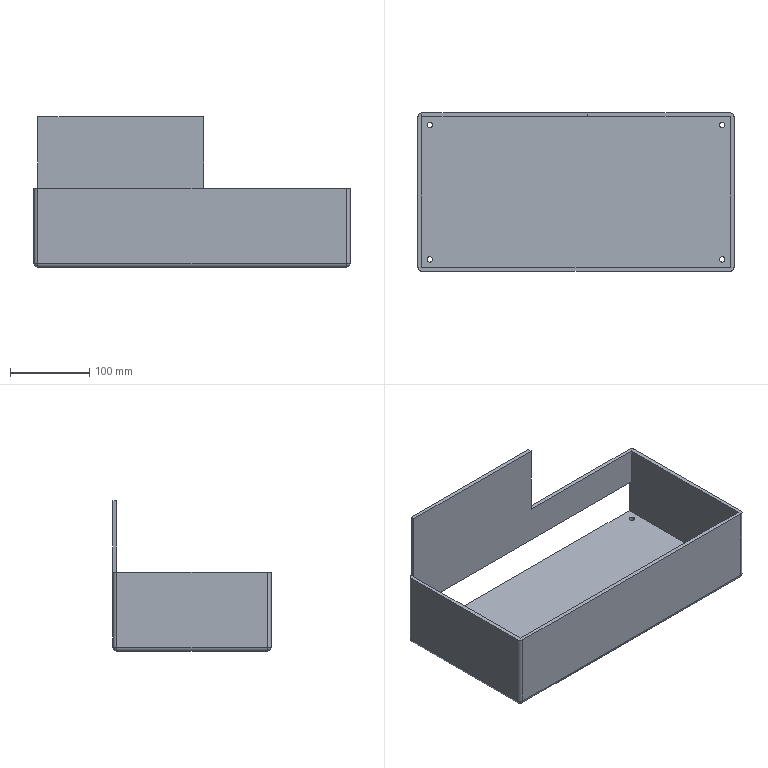Part | SolidWorks | features ICE 3, Fillet 2, Extrusion 1, Shell 1 | 1 solid | 35 faces | box 400 x 200 x 190 mm | volume 953105 mm3 | cylinder 16 | plane 15 | sphere 4 | commonest cylinder face diameters 7 x8 10 x8
STEP:
#1=CARTESIAN_POINT('',(-188.5,-85.,0.));
#2=VERTEX_POINT('',#1);
#3=CARTESIAN_POINT('',(-181.5,-85.,0.));
#4=VERTEX_POINT('',#3);
#5=CARTESIAN_POINT('',(-185.,-85.,0.));
#6=DIRECTION('',(0.,0.,1.));
#7=DIRECTION('',(1.,0.,0.));
#8=AXIS2_PLACEMENT_3D('',#5,#6,#7);
#9=CIRCLE('',#8,3.5);
#10=EDGE_CURVE('',#2,#4,#9,.T.);
#11=ORIENTED_EDGE('',*,*,#10,.F.);
#12=CARTESIAN_POINT('',(-188.5,-85.,5.));
#13=VERTEX_POINT('',#12);
#14=CARTESIAN_POINT('',(-188.5,-85.,-55.));
#15=DIRECTION('',(0.,0.,1.));
#16=VECTOR('',#15,1000.);
#17=LINE('',#14,#16);
#18=EDGE_CURVE('',#2,#13,#17,.T.);
#19=ORIENTED_EDGE('',*,*,#18,.T.);
#20=CARTESIAN_POINT('',(-181.5,-85.,5.));
#21=VERTEX_POINT('',#20);
#22=CARTESIAN_POINT('',(-185.,-85.,5.));
#23=DIRECTION('',(0.,0.,1.));
#24=DIRECTION('',(-1.,0.,0.));
#25=AXIS2_PLACEMENT_3D('',#22,#23,#24);
#26=CIRCLE('',#25,3.5);
#27=EDGE_CURVE('',#13,#21,#26,.T.);
#28=ORIENTED_EDGE('',*,*,#27,.T.);
#29=CARTESIAN_POINT('',(-181.5,-85.,-55.));
#30=DIRECTION('',(0.,0.,1.));
#31=VECTOR('',#30,1000.);
#32=LINE('',#29,#31);
#33=EDGE_CURVE('',#4,#21,#32,.T.);
#34=ORIENTED_EDGE('',*,*,#33,.F.);
#35=EDGE_LOOP('',(#11,#19,#28,#34));
#36=FACE_OUTER_BOUND('',#35,.T.);
#37=CARTESIAN_POINT('',(-185.,-85.,-55.));
#38=DIRECTION('',(0.,0.,1.));
#39=DIRECTION('',(1.,0.,0.));
#40=AXIS2_PLACEMENT_3D('',#37,#38,#39);
#41=CYLINDRICAL_SURFACE('',#40,3.5);
#42=ADVANCED_FACE('',(#36),#41,.F.);
#43=CARTESIAN_POINT('',(181.5,-85.,0.));
#44=VERTEX_POINT('',#43);
#45=CARTESIAN_POINT('',(188.5,-85.,0.));
#46=VERTEX_POINT('',#45);
#47=CARTESIAN_POINT('',(185.,-85.,0.));
#48=DIRECTION('',(0.,0.,1.));
#49=DIRECTION('',(1.,0.,0.));
#50=AXIS2_PLACEMENT_3D('',#47,#48,#49);
#51=CIRCLE('',#50,3.5);
#52=EDGE_CURVE('',#44,#46,#51,.T.);
#53=ORIENTED_EDGE('',*,*,#52,.F.);
#54=CARTESIAN_POINT('',(181.5,-85.,5.));
#55=VERTEX_POINT('',#54);
#56=CARTESIAN_POINT('',(181.5,-85.,-55.));
#57=DIRECTION('',(0.,0.,1.));
#58=VECTOR('',#57,1000.);
#59=LINE('',#56,#58);
#60=EDGE_CURVE('',#44,#55,#59,.T.);
#61=ORIENTED_EDGE('',*,*,#60,.T.);
#62=CARTESIAN_POINT('',(188.5,-85.,5.));
#63=VERTEX_POINT('',#62);
#64=CARTESIAN_POINT('',(185.,-85.,5.));
#65=DIRECTION('',(0.,0.,1.));
#66=DIRECTION('',(1.,0.,0.));
#67=AXIS2_PLACEMENT_3D('',#64,#65,#66);
#68=CIRCLE('',#67,3.5);
#69=EDGE_CURVE('',#55,#63,#68,.T.);
#70=ORIENTED_EDGE('',*,*,#69,.T.);
#71=CARTESIAN_POINT('',(188.5,-85.,-55.));
#72=DIRECTION('',(0.,0.,1.));
#73=VECTOR('',#72,1000.);
#74=LINE('',#71,#73);
#75=EDGE_CURVE('',#46,#63,#74,.T.);
#76=ORIENTED_EDGE('',*,*,#75,.F.);
#77=EDGE_LOOP('',(#53,#61,#70,#76));
#78=FACE_OUTER_BOUND('',#77,.T.);
#79=CARTESIAN_POINT('',(185.,-85.,-55.));
#80=DIRECTION('',(0.,0.,1.));
#81=DIRECTION('',(1.,0.,0.));
#82=AXIS2_PLACEMENT_3D('',#79,#80,#81);
#83=CYLINDRICAL_SURFACE('',#82,3.5);
#84=ADVANCED_FACE('',(#78),#83,.F.);
#85=CARTESIAN_POINT('',(181.5,85.,0.));
#86=VERTEX_POINT('',#85);
#87=CARTESIAN_POINT('',(188.5,85.,0.));
#88=VERTEX_POINT('',#87);
#89=CARTESIAN_POINT('',(185.,85.,0.));
#90=DIRECTION('',(0.,0.,1.));
#91=DIRECTION('',(1.,0.,0.));
#92=AXIS2_PLACEMENT_3D('',#89,#90,#91);
#93=CIRCLE('',#92,3.5);
#94=EDGE_CURVE('',#86,#88,#93,.T.);
#95=ORIENTED_EDGE('',*,*,#94,.F.);
#96=CARTESIAN_POINT('',(181.5,85.,5.));
#97=VERTEX_POINT('',#96);
#98=CARTESIAN_POINT('',(181.5,85.,-55.));
#99=DIRECTION('',(0.,0.,1.));
#100=VECTOR('',#99,1000.);
#101=LINE('',#98,#100);
#102=EDGE_CURVE('',#86,#97,#101,.T.);
#103=ORIENTED_EDGE('',*,*,#102,.T.);
#104=CARTESIAN_POINT('',(188.5,85.,5.));
#105=VERTEX_POINT('',#104);
#106=CARTESIAN_POINT('',(185.,85.,5.));
#107=DIRECTION('',(0.,0.,1.));
#108=DIRECTION('',(-1.,0.,0.));
#109=AXIS2_PLACEMENT_3D('',#106,#107,#108);
#110=CIRCLE('',#109,3.5);
#111=EDGE_CURVE('',#97,#105,#110,.T.);
#112=ORIENTED_EDGE('',*,*,#111,.T.);
#113=CARTESIAN_POINT('',(188.5,85.,-55.));
#114=DIRECTION('',(0.,0.,1.));
#115=VECTOR('',#114,1000.);
#116=LINE('',#113,#115);
#117=EDGE_CURVE('',#88,#105,#116,.T.);
#118=ORIENTED_EDGE('',*,*,#117,.F.);
#119=EDGE_LOOP('',(#95,#103,#112,#118));
#120=FACE_OUTER_BOUND('',#119,.T.);
#121=CARTESIAN_POINT('',(185.,85.,-55.));
#122=DIRECTION('',(0.,0.,1.));
#123=DIRECTION('',(1.,0.,0.));
#124=AXIS2_PLACEMENT_3D('',#121,#122,#123);
#125=CYLINDRICAL_SURFACE('',#124,3.5);
#126=ADVANCED_FACE('',(#120),#125,.F.);
#127=CARTESIAN_POINT('',(-188.5,85.,0.));
#128=VERTEX_POINT('',#127);
#129=CARTESIAN_POINT('',(-181.5,85.,0.));
#130=VERTEX_POINT('',#129);
#131=CARTESIAN_POINT('',(-185.,85.,0.));
#132=DIRECTION('',(0.,0.,1.));
#133=DIRECTION('',(1.,0.,0.));
#134=AXIS2_PLACEMENT_3D('',#131,#132,#133);
#135=CIRCLE('',#134,3.5);
#136=EDGE_CURVE('',#128,#130,#135,.T.);
#137=ORIENTED_EDGE('',*,*,#136,.F.);
#138=CARTESIAN_POINT('',(-188.5,85.,5.));
#139=VERTEX_POINT('',#138);
#140=CARTESIAN_POINT('',(-188.5,85.,-55.));
#141=DIRECTION('',(0.,0.,1.));
#142=VECTOR('',#141,1000.);
#143=LINE('',#140,#142);
#144=EDGE_CURVE('',#128,#139,#143,.T.);
#145=ORIENTED_EDGE('',*,*,#144,.T.);
#146=CARTESIAN_POINT('',(-181.5,85.,5.));
#147=VERTEX_POINT('',#146);
#148=CARTESIAN_POINT('',(-185.,85.,5.));
#149=DIRECTION('',(0.,0.,1.));
#150=DIRECTION('',(1.,0.,0.));
#151=AXIS2_PLACEMENT_3D('',#148,#149,#150);
#152=CIRCLE('',#151,3.5);
#153=EDGE_CURVE('',#139,#147,#152,.T.);
#154=ORIENTED_EDGE('',*,*,#153,.T.);
#155=CARTESIAN_POINT('',(-181.5,85.,-55.));
#156=DIRECTION('',(0.,0.,1.));
#157=VECTOR('',#156,1000.);
#158=LINE('',#155,#157);
#159=EDGE_CURVE('',#130,#147,#158,.T.);
#160=ORIENTED_EDGE('',*,*,#159,.F.);
#161=EDGE_LOOP('',(#137,#145,#154,#160));
#162=FACE_OUTER_BOUND('',#161,.T.);
#163=CARTESIAN_POINT('',(-185.,85.,-55.));
#164=DIRECTION('',(0.,0.,1.));
#165=DIRECTION('',(1.,0.,0.));
#166=AXIS2_PLACEMENT_3D('',#163,#164,#165);
#167=CYLINDRICAL_SURFACE('',#166,3.5);
#168=ADVANCED_FACE('',(#162),#167,.F.);
#169=CARTESIAN_POINT('',(-195.,100.,52.5));
#170=VERTEX_POINT('',#169);
#171=CARTESIAN_POINT('',(195.,100.,52.5));
#172=VERTEX_POINT('',#171);
#173=CARTESIAN_POINT('',(-195.,100.,52.5));
#174=DIRECTION('',(1.,0.,0.));
#175=VECTOR('',#174,1000.);
#176=LINE('',#173,#175);
#177=EDGE_CURVE('',#170,#172,#176,.T.);
#178=ORIENTED_EDGE('',*,*,#177,.F.);
#179=CARTESIAN_POINT('',(-195.,100.,100.));
#180=VERTEX_POINT('',#179);
#181=CARTESIAN_POINT('',(-195.,100.,100.));
#182=DIRECTION('',(0.,0.,1.));
#183=VECTOR('',#182,1000.);
#184=LINE('',#181,#183);
#185=EDGE_CURVE('',#170,#180,#184,.T.);
#186=ORIENTED_EDGE('',*,*,#185,.T.);
#187=CARTESIAN_POINT('',(-195.,100.,190.));
#188=VERTEX_POINT('',#187);
#189=CARTESIAN_POINT('',(-195.,100.,100.));
#190=DIRECTION('',(0.,0.,1.));
#191=VECTOR('',#190,1000.);
#192=LINE('',#189,#191);
#193=EDGE_CURVE('',#180,#188,#192,.T.);
#194=ORIENTED_EDGE('',*,*,#193,.T.);
#195=CARTESIAN_POINT('',(15.,100.,190.));
#196=VERTEX_POINT('',#195);
#197=CARTESIAN_POINT('',(-195.,100.,190.));
#198=DIRECTION('',(1.,0.,0.));
#199=VECTOR('',#198,1000.);
#200=LINE('',#197,#199);
#201=EDGE_CURVE('',#188,#196,#200,.T.);
#202=ORIENTED_EDGE('',*,*,#201,.T.);
#203=CARTESIAN_POINT('',(15.,100.,100.));
#204=VERTEX_POINT('',#203);
#205=CARTESIAN_POINT('',(15.,100.,100.));
#206=DIRECTION('',(0.,0.,-1.));
#207=VECTOR('',#206,1000.);
#208=LINE('',#205,#207);
#209=EDGE_CURVE('',#196,#204,#208,.T.);
#210=ORIENTED_EDGE('',*,*,#209,.T.);
#211=CARTESIAN_POINT('',(195.,100.,100.));
#212=VERTEX_POINT('',#211);
#213=CARTESIAN_POINT('',(-200.,100.,100.));
#214=DIRECTION('',(-1.,0.,0.));
#215=VECTOR('',#214,1000.);
#216=LINE('',#213,#215);
#217=EDGE_CURVE('',#212,#204,#216,.T.);
#218=ORIENTED_EDGE('',*,*,#217,.F.);
#219=CARTESIAN_POINT('',(195.,100.,100.));
#220=DIRECTION('',(0.,0.,-1.));
#221=VECTOR('',#220,1000.);
#222=LINE('',#219,#221);
#223=EDGE_CURVE('',#212,#172,#222,.T.);
#224=ORIENTED_EDGE('',*,*,#223,.T.);
#225=EDGE_LOOP('',(#178,#186,#194,#202,#210,#218,#224));
#226=FACE_OUTER_BOUND('',#225,.T.);
#227=CARTESIAN_POINT('',(-200.,100.,100.));
#228=DIRECTION('',(0.,-1.,0.));
#229=DIRECTION('',(0.,0.,-1.));
#230=AXIS2_PLACEMENT_3D('',#227,#228,#229);
#231=PLANE('',#230);
#232=ADVANCED_FACE('',(#226),#231,.F.);
#233=CARTESIAN_POINT('',(-195.,95.,100.));
#234=VERTEX_POINT('',#233);
#235=CARTESIAN_POINT('',(-195.,95.,52.5));
#236=VERTEX_POINT('',#235);
#237=CARTESIAN_POINT('',(-195.,95.,100.));
#238=DIRECTION('',(0.,0.,-1.));
#239=VECTOR('',#238,1000.);
#240=LINE('',#237,#239);
#241=EDGE_CURVE('',#234,#236,#240,.T.);
#242=ORIENTED_EDGE('',*,*,#241,.T.);
#243=CARTESIAN_POINT('',(195.,95.,52.5));
#244=VERTEX_POINT('',#243);
#245=CARTESIAN_POINT('',(-200.,95.,52.5));
#246=DIRECTION('',(1.,0.,0.));
#247=VECTOR('',#246,1000.);
#248=LINE('',#245,#247);
#249=EDGE_CURVE('',#236,#244,#248,.T.);
#250=ORIENTED_EDGE('',*,*,#249,.T.);
#251=CARTESIAN_POINT('',(195.,95.,100.));
#252=VERTEX_POINT('',#251);
#253=CARTESIAN_POINT('',(195.,95.,100.));
#254=DIRECTION('',(0.,0.,-1.));
#255=VECTOR('',#254,1000.);
#256=LINE('',#253,#255);
#257=EDGE_CURVE('',#252,#244,#256,.T.);
#258=ORIENTED_EDGE('',*,*,#257,.F.);
#259=CARTESIAN_POINT('',(15.,95.,100.));
#260=VERTEX_POINT('',#259);
#261=CARTESIAN_POINT('',(-200.,95.,100.));
#262=DIRECTION('',(-1.,0.,0.));
#263=VECTOR('',#262,1000.);
#264=LINE('',#261,#263);
#265=EDGE_CURVE('',#252,#260,#264,.T.);
#266=ORIENTED_EDGE('',*,*,#265,.T.);
#267=CARTESIAN_POINT('',(15.,95.,190.));
#268=VERTEX_POINT('',#267);
#269=CARTESIAN_POINT('',(15.,95.,100.));
#270=DIRECTION('',(0.,0.,-1.));
#271=VECTOR('',#270,1000.);
#272=LINE('',#269,#271);
#273=EDGE_CURVE('',#268,#260,#272,.T.);
#274=ORIENTED_EDGE('',*,*,#273,.F.);
#275=CARTESIAN_POINT('',(-195.,95.,190.));
#276=VERTEX_POINT('',#275);
#277=CARTESIAN_POINT('',(-195.,95.,190.));
#278=DIRECTION('',(1.,0.,0.));
#279=VECTOR('',#278,1000.);
#280=LINE('',#277,#279);
#281=EDGE_CURVE('',#276,#268,#280,.T.);
#282=ORIENTED_EDGE('',*,*,#281,.F.);
#283=CARTESIAN_POINT('',(-195.,95.,100.));
#284=DIRECTION('',(0.,0.,1.));
#285=VECTOR('',#284,1000.);
#286=LINE('',#283,#285);
#287=EDGE_CURVE('',#234,#276,#286,.T.);
#288=ORIENTED_EDGE('',*,*,#287,.F.);
#289=EDGE_LOOP('',(#242,#250,#258,#266,#274,#282,#288));
#290=FACE_OUTER_BOUND('',#289,.T.);
#291=CARTESIAN_POINT('',(-200.,95.,100.));
#292=DIRECTION('',(0.,-1.,0.));
#293=DIRECTION('',(0.,0.,-1.));
#294=AXIS2_PLACEMENT_3D('',#291,#292,#293);
#295=PLANE('',#294);
#296=ADVANCED_FACE('',(#290),#295,.T.);
#297=CARTESIAN_POINT('',(200.,-95.,100.));
#298=VERTEX_POINT('',#297);
#299=CARTESIAN_POINT('',(200.,-95.,5.));
#300=VERTEX_POINT('',#299);
#301=CARTESIAN_POINT('',(200.,-95.,100.));
#302=DIRECTION('',(0.,0.,-1.));
#303=VECTOR('',#302,1000.);
#304=LINE('',#301,#303);
#305=EDGE_CURVE('',#298,#300,#304,.T.);
#306=ORIENTED_EDGE('',*,*,#305,.T.);
#307=CARTESIAN_POINT('',(200.,95.,5.));
#308=VERTEX_POINT('',#307);
#309=CARTESIAN_POINT('',(200.,100.,5.));
#310=DIRECTION('',(0.,1.,0.));
#311=VECTOR('',#310,1000.);
#312=LINE('',#309,#311);
#313=EDGE_CURVE('',#300,#308,#312,.T.);
#314=ORIENTED_EDGE('',*,*,#313,.T.);
#315=CARTESIAN_POINT('',(200.,95.,100.));
#316=VERTEX_POINT('',#315);
#317=CARTESIAN_POINT('',(200.,95.,100.));
#318=DIRECTION('',(0.,0.,1.));
#319=VECTOR('',#318,1000.);
#320=LINE('',#317,#319);
#321=EDGE_CURVE('',#308,#316,#320,.T.);
#322=ORIENTED_EDGE('',*,*,#321,.T.);
#323=CARTESIAN_POINT('',(200.,100.,100.));
#324=DIRECTION('',(0.,1.,0.));
#325=VECTOR('',#324,1000.);
#326=LINE('',#323,#325);
#327=EDGE_CURVE('',#298,#316,#326,.T.);
#328=ORIENTED_EDGE('',*,*,#327,.F.);
#329=EDGE_LOOP('',(#306,#314,#322,#328));
#330=FACE_OUTER_BOUND('',#329,.T.);
#331=CARTESIAN_POINT('',(200.,100.,100.));
#332=DIRECTION('',(-1.,0.,0.));
#333=DIRECTION('',(0.,-1.,0.));
#334=AXIS2_PLACEMENT_3D('',#331,#332,#333);
#335=PLANE('',#334);
#336=ADVANCED_FACE('',(#330),#335,.F.);
#337=CARTESIAN_POINT('',(-200.,95.,100.));
#338=VERTEX_POINT('',#337);
#339=CARTESIAN_POINT('',(-200.,95.,5.));
#340=VERTEX_POINT('',#339);
#341=CARTESIAN_POINT('',(-200.,95.,100.));
#342=DIRECTION('',(0.,0.,-1.));
#343=VECTOR('',#342,1000.);
#344=LINE('',#341,#343);
#345=EDGE_CURVE('',#338,#340,#344,.T.);
#346=ORIENTED_EDGE('',*,*,#345,.T.);
#347=CARTESIAN_POINT('',(-200.,-95.,5.));
#348=VERTEX_POINT('',#347);
#349=CARTESIAN_POINT('',(-200.,100.,5.));
#350=DIRECTION('',(0.,-1.,0.));
#351=VECTOR('',#350,1000.);
#352=LINE('',#349,#351);
#353=EDGE_CURVE('',#340,#348,#352,.T.);
#354=ORIENTED_EDGE('',*,*,#353,.T.);
#355=CARTESIAN_POINT('',(-200.,-95.,100.));
#356=VERTEX_POINT('',#355);
#357=CARTESIAN_POINT('',(-200.,-95.,100.));
#358=DIRECTION('',(0.,0.,1.));
#359=VECTOR('',#358,1000.);
#360=LINE('',#357,#359);
#361=EDGE_CURVE('',#348,#356,#360,.T.);
#362=ORIENTED_EDGE('',*,*,#361,.T.);
#363=CARTESIAN_POINT('',(-200.,100.,100.));
#364=DIRECTION('',(0.,-1.,0.));
#365=VECTOR('',#364,1000.);
#366=LINE('',#363,#365);
#367=EDGE_CURVE('',#338,#356,#366,.T.);
#368=ORIENTED_EDGE('',*,*,#367,.F.);
#369=EDGE_LOOP('',(#346,#354,#362,#368));
#370=FACE_OUTER_BOUND('',#369,.T.);
#371=CARTESIAN_POINT('',(-200.,100.,100.));
#372=DIRECTION('',(1.,0.,0.));
#373=DIRECTION('',(0.,1.,0.));
#374=AXIS2_PLACEMENT_3D('',#371,#372,#373);
#375=PLANE('',#374);
#376=ADVANCED_FACE('',(#370),#375,.F.);
#377=CARTESIAN_POINT('',(-195.,-100.,100.));
#378=VERTEX_POINT('',#377);
#379=CARTESIAN_POINT('',(-195.,-100.,5.));
#380=VERTEX_POINT('',#379);
#381=CARTESIAN_POINT('',(-195.,-100.,100.));
#382=DIRECTION('',(0.,0.,-1.));
#383=VECTOR('',#382,1000.);
#384=LINE('',#381,#383);
#385=EDGE_CURVE('',#378,#380,#384,.T.);
#386=ORIENTED_EDGE('',*,*,#385,.T.);
#387=CARTESIAN_POINT('',(195.,-100.,5.));
#388=VERTEX_POINT('',#387);
#389=CARTESIAN_POINT('',(-200.,-100.,5.));
#390=DIRECTION('',(1.,0.,0.));
#391=VECTOR('',#390,1000.);
#392=LINE('',#389,#391);
#393=EDGE_CURVE('',#380,#388,#392,.T.);
#394=ORIENTED_EDGE('',*,*,#393,.T.);
#395=CARTESIAN_POINT('',(195.,-100.,100.));
#396=VERTEX_POINT('',#395);
#397=CARTESIAN_POINT('',(195.,-100.,100.));
#398=DIRECTION('',(0.,0.,1.));
#399=VECTOR('',#398,1000.);
#400=LINE('',#397,#399);
#401=EDGE_CURVE('',#388,#396,#400,.T.);
#402=ORIENTED_EDGE('',*,*,#401,.T.);
#403=CARTESIAN_POINT('',(-200.,-100.,100.));
#404=DIRECTION('',(1.,0.,0.));
#405=VECTOR('',#404,1000.);
#406=LINE('',#403,#405);
#407=EDGE_CURVE('',#378,#396,#406,.T.);
#408=ORIENTED_EDGE('',*,*,#407,.F.);
#409=EDGE_LOOP('',(#386,#394,#402,#408));
#410=FACE_OUTER_BOUND('',#409,.T.);
#411=CARTESIAN_POINT('',(-200.,-100.,100.));
#412=DIRECTION('',(0.,1.,0.));
#413=DIRECTION('',(0.,0.,1.));
#414=AXIS2_PLACEMENT_3D('',#411,#412,#413);
#415=PLANE('',#414);
#416=ADVANCED_FACE('',(#410),#415,.F.);
#417=CARTESIAN_POINT('',(15.,-133.473,100.));
#418=DIRECTION('',(0.,1.,0.));
#419=VECTOR('',#418,1000.);
#420=LINE('',#417,#419);
#421=EDGE_CURVE('',#260,#204,#420,.T.);
#422=ORIENTED_EDGE('',*,*,#421,.F.);
#423=ORIENTED_EDGE('',*,*,#265,.F.);
#424=CARTESIAN_POINT('',(195.,-95.,100.));
#425=VERTEX_POINT('',#424);
#426=CARTESIAN_POINT('',(195.,100.,100.));
#427=DIRECTION('',(0.,1.,0.));
#428=VECTOR('',#427,1000.);
#429=LINE('',#426,#428);
#430=EDGE_CURVE('',#425,#252,#429,.T.);
#431=ORIENTED_EDGE('',*,*,#430,.F.);
#432=CARTESIAN_POINT('',(-195.,-95.,100.));
#433=VERTEX_POINT('',#432);
#434=CARTESIAN_POINT('',(-200.,-95.,100.));
#435=DIRECTION('',(1.,0.,0.));
#436=VECTOR('',#435,1000.);
#437=LINE('',#434,#436);
#438=EDGE_CURVE('',#433,#425,#437,.T.);
#439=ORIENTED_EDGE('',*,*,#438,.F.);
#440=CARTESIAN_POINT('',(-195.,100.,100.));
#441=DIRECTION('',(0.,-1.,0.));
#442=VECTOR('',#441,1000.);
#443=LINE('',#440,#442);
#444=EDGE_CURVE('',#234,#433,#443,.T.);
#445=ORIENTED_EDGE('',*,*,#444,.F.);
#446=CARTESIAN_POINT('',(-195.,-133.473,100.));
#447=DIRECTION('',(0.,1.,0.));
#448=VECTOR('',#447,1000.);
#449=LINE('',#446,#448);
#450=EDGE_CURVE('',#234,#180,#449,.T.);
#451=ORIENTED_EDGE('',*,*,#450,.T.);
#452=CARTESIAN_POINT('',(-195.,95.,100.));
#453=DIRECTION('',(0.,0.,1.));
#454=DIRECTION('',(1.,0.,0.));
#455=AXIS2_PLACEMENT_3D('',#452,#453,#454);
#456=CIRCLE('',#455,5.);
#457=EDGE_CURVE('',#180,#338,#456,.T.);
#458=ORIENTED_EDGE('',*,*,#457,.T.);
#459=ORIENTED_EDGE('',*,*,#367,.T.);
#460=CARTESIAN_POINT('',(-195.,-95.,100.));
#461=DIRECTION('',(0.,0.,1.));
#462=DIRECTION('',(1.,0.,0.));
#463=AXIS2_PLACEMENT_3D('',#460,#461,#462);
#464=CIRCLE('',#463,5.);
#465=EDGE_CURVE('',#356,#378,#464,.T.);
#466=ORIENTED_EDGE('',*,*,#465,.T.);
#467=ORIENTED_EDGE('',*,*,#407,.T.);
#468=CARTESIAN_POINT('',(195.,-95.,100.));
#469=DIRECTION('',(0.,0.,1.));
#470=DIRECTION('',(1.,0.,0.));
#471=AXIS2_PLACEMENT_3D('',#468,#469,#470);
#472=CIRCLE('',#471,5.);
#473=EDGE_CURVE('',#396,#298,#472,.T.);
#474=ORIENTED_EDGE('',*,*,#473,.T.);
#475=ORIENTED_EDGE('',*,*,#327,.T.);
#476=CARTESIAN_POINT('',(195.,95.,100.));
#477=DIRECTION('',(0.,0.,1.));
#478=DIRECTION('',(1.,0.,0.));
#479=AXIS2_PLACEMENT_3D('',#476,#477,#478);
#480=CIRCLE('',#479,5.);
#481=EDGE_CURVE('',#316,#212,#480,.T.);
#482=ORIENTED_EDGE('',*,*,#481,.T.);
#483=ORIENTED_EDGE('',*,*,#217,.T.);
#484=EDGE_LOOP('',(#422,#423,#431,#439,#445,#451,#458,#459,#466,#467,#474,#475,#482,#483));
#485=FACE_OUTER_BOUND('',#484,.T.);
#486=CARTESIAN_POINT('',(0.,0.,100.));
#487=DIRECTION('',(0.,0.,1.));
#488=DIRECTION('',(1.,0.,0.));
#489=AXIS2_PLACEMENT_3D('',#486,#487,#488);
#490=PLANE('',#489);
#491=ADVANCED_FACE('',(#485),#490,.T.);
#492=CARTESIAN_POINT('',(-185.,-85.,0.));
#493=DIRECTION('',(0.,0.,1.));
#494=DIRECTION('',(1.,0.,0.));
#495=AXIS2_PLACEMENT_3D('',#492,#493,#494);
#496=CIRCLE('',#495,3.5);
#497=EDGE_CURVE('',#4,#2,#496,.T.);
#498=ORIENTED_EDGE('',*,*,#497,.T.);
#499=ORIENTED_EDGE('',*,*,#10,.T.);
#500=EDGE_LOOP('',(#498,#499));
#501=FACE_BOUND('',#500,.T.);
#502=CARTESIAN_POINT('',(185.,-85.,0.));
#503=DIRECTION('',(0.,0.,1.));
#504=DIRECTION('',(1.,0.,0.));
#505=AXIS2_PLACEMENT_3D('',#502,#503,#504);
#506=CIRCLE('',#505,3.5);
#507=EDGE_CURVE('',#46,#44,#506,.T.);
#508=ORIENTED_EDGE('',*,*,#507,.T.);
#509=ORIENTED_EDGE('',*,*,#52,.T.);
#510=EDGE_LOOP('',(#508,#509));
#511=FACE_BOUND('',#510,.T.);
#512=CARTESIAN_POINT('',(185.,85.,0.));
#513=DIRECTION('',(0.,0.,1.));
#514=DIRECTION('',(1.,0.,0.));
#515=AXIS2_PLACEMENT_3D('',#512,#513,#514);
#516=CIRCLE('',#515,3.5);
#517=EDGE_CURVE('',#88,#86,#516,.T.);
#518=ORIENTED_EDGE('',*,*,#517,.T.);
#519=ORIENTED_EDGE('',*,*,#94,.T.);
#520=EDGE_LOOP('',(#518,#519));
#521=FACE_BOUND('',#520,.T.);
#522=CARTESIAN_POINT('',(-185.,85.,0.));
#523=DIRECTION('',(0.,0.,1.));
#524=DIRECTION('',(1.,0.,0.));
#525=AXIS2_PLACEMENT_3D('',#522,#523,#524);
#526=CIRCLE('',#525,3.5);
#527=EDGE_CURVE('',#130,#128,#526,.T.);
#528=ORIENTED_EDGE('',*,*,#527,.T.);
#529=ORIENTED_EDGE('',*,*,#136,.T.);
#530=EDGE_LOOP('',(#528,#529));
#531=FACE_BOUND('',#530,.T.);
#532=CARTESIAN_POINT('',(195.,-95.,0.));
#533=VERTEX_POINT('',#532);
#534=CARTESIAN_POINT('',(-195.,-95.,0.));
#535=VERTEX_POINT('',#534);
#536=CARTESIAN_POINT('',(0.,-95.,0.));
#537=DIRECTION('',(-1.,0.,0.));
#538=VECTOR('',#537,1000.);
#539=LINE('',#536,#538);
#540=EDGE_CURVE('',#533,#535,#539,.T.);
#541=ORIENTED_EDGE('',*,*,#540,.T.);
#542=CARTESIAN_POINT('',(-195.,95.,0.));
#543=VERTEX_POINT('',#542);
#544=CARTESIAN_POINT('',(-195.,0.,0.));
#545=DIRECTION('',(0.,1.,0.));
#546=VECTOR('',#545,1000.);
#547=LINE('',#544,#546);
#548=EDGE_CURVE('',#535,#543,#547,.T.);
#549=ORIENTED_EDGE('',*,*,#548,.T.);
#550=CARTESIAN_POINT('',(195.,95.,0.));
#551=VERTEX_POINT('',#550);
#552=CARTESIAN_POINT('',(0.,95.,0.));
#553=DIRECTION('',(1.,0.,0.));
#554=VECTOR('',#553,1000.);
#555=LINE('',#552,#554);
#556=EDGE_CURVE('',#543,#551,#555,.T.);
#557=ORIENTED_EDGE('',*,*,#556,.T.);
#558=CARTESIAN_POINT('',(195.,0.,0.));
#559=DIRECTION('',(0.,-1.,0.));
#560=VECTOR('',#559,1000.);
#561=LINE('',#558,#560);
#562=EDGE_CURVE('',#551,#533,#561,.T.);
#563=ORIENTED_EDGE('',*,*,#562,.T.);
#564=EDGE_LOOP('',(#541,#549,#557,#563));
#565=FACE_OUTER_BOUND('',#564,.T.);
#566=CARTESIAN_POINT('',(0.,0.,0.));
#567=DIRECTION('',(0.,0.,1.));
#568=DIRECTION('',(1.,0.,0.));
#569=AXIS2_PLACEMENT_3D('',#566,#567,#568);
#570=PLANE('',#569);
#571=ADVANCED_FACE('',(#501,#511,#521,#531,#565),#570,.F.);
#572=ORIENTED_EDGE('',*,*,#401,.F.);
#573=CARTESIAN_POINT('',(195.,-95.,5.));
#574=DIRECTION('',(0.,0.,1.));
#575=DIRECTION('',(-1.,0.,0.));
#576=AXIS2_PLACEMENT_3D('',#573,#574,#575);
#577=CIRCLE('',#576,5.);
#578=EDGE_CURVE('',#388,#300,#577,.T.);
#579=ORIENTED_EDGE('',*,*,#578,.T.);
#580=ORIENTED_EDGE('',*,*,#305,.F.);
#581=ORIENTED_EDGE('',*,*,#473,.F.);
#582=EDGE_LOOP('',(#572,#579,#580,#581));
#583=FACE_OUTER_BOUND('',#582,.T.);
#584=CARTESIAN_POINT('',(195.,-95.,100.));
#585=DIRECTION('',(0.,0.,-1.));
#586=DIRECTION('',(-1.,0.,0.));
#587=AXIS2_PLACEMENT_3D('',#584,#585,#586);
#588=CYLINDRICAL_SURFACE('',#587,5.);
#589=ADVANCED_FACE('',(#583),#588,.T.);
#590=ORIENTED_EDGE('',*,*,#321,.F.);
#591=CARTESIAN_POINT('',(195.,100.,5.));
#592=VERTEX_POINT('',#591);
#593=CARTESIAN_POINT('',(195.,95.,5.));
#594=DIRECTION('',(0.,0.,1.));
#595=DIRECTION('',(-1.,0.,0.));
#596=AXIS2_PLACEMENT_3D('',#593,#594,#595);
#597=CIRCLE('',#596,5.);
#598=EDGE_CURVE('',#308,#592,#597,.T.);
#599=ORIENTED_EDGE('',*,*,#598,.T.);
#600=CARTESIAN_POINT('',(195.,100.,52.5));
#601=DIRECTION('',(0.,0.,-1.));
#602=VECTOR('',#601,1000.);
#603=LINE('',#600,#602);
#604=EDGE_CURVE('',#172,#592,#603,.T.);
#605=ORIENTED_EDGE('',*,*,#604,.F.);
#606=ORIENTED_EDGE('',*,*,#223,.F.);
#607=ORIENTED_EDGE('',*,*,#481,.F.);
#608=EDGE_LOOP('',(#590,#599,#605,#606,#607));
#609=FACE_OUTER_BOUND('',#608,.T.);
#610=CARTESIAN_POINT('',(195.,95.,100.));
#611=DIRECTION('',(0.,0.,-1.));
#612=DIRECTION('',(-1.,0.,0.));
#613=AXIS2_PLACEMENT_3D('',#610,#611,#612);
#614=CYLINDRICAL_SURFACE('',#613,5.);
#615=ADVANCED_FACE('',(#609),#614,.T.);
#616=CARTESIAN_POINT('',(-195.,100.,5.));
#617=VERTEX_POINT('',#616);
#618=CARTESIAN_POINT('',(-195.,100.,100.));
#619=DIRECTION('',(0.,0.,1.));
#620=VECTOR('',#619,1000.);
#621=LINE('',#618,#620);
#622=EDGE_CURVE('',#617,#170,#621,.T.);
#623=ORIENTED_EDGE('',*,*,#622,.F.);
#624=CARTESIAN_POINT('',(-195.,95.,5.));
#625=DIRECTION('',(0.,0.,1.));
#626=DIRECTION('',(-1.,0.,0.));
#627=AXIS2_PLACEMENT_3D('',#624,#625,#626);
#628=CIRCLE('',#627,5.);
#629=EDGE_CURVE('',#617,#340,#628,.T.);
#630=ORIENTED_EDGE('',*,*,#629,.T.);
#631=ORIENTED_EDGE('',*,*,#345,.F.);
#632=ORIENTED_EDGE('',*,*,#457,.F.);
#633=ORIENTED_EDGE('',*,*,#185,.F.);
#634=EDGE_LOOP('',(#623,#630,#631,#632,#633));
#635=FACE_OUTER_BOUND('',#634,.T.);
#636=CARTESIAN_POINT('',(-195.,95.,100.));
#637=DIRECTION('',(0.,0.,-1.));
#638=DIRECTION('',(-1.,0.,0.));
#639=AXIS2_PLACEMENT_3D('',#636,#637,#638);
#640=CYLINDRICAL_SURFACE('',#639,5.);
#641=ADVANCED_FACE('',(#635),#640,.T.);
#642=ORIENTED_EDGE('',*,*,#361,.F.);
#643=CARTESIAN_POINT('',(-195.,-95.,5.));
#644=DIRECTION('',(0.,0.,1.));
#645=DIRECTION('',(-1.,0.,0.));
#646=AXIS2_PLACEMENT_3D('',#643,#644,#645);
#647=CIRCLE('',#646,5.);
#648=EDGE_CURVE('',#348,#380,#647,.T.);
#649=ORIENTED_EDGE('',*,*,#648,.T.);
#650=ORIENTED_EDGE('',*,*,#385,.F.);
#651=ORIENTED_EDGE('',*,*,#465,.F.);
#652=EDGE_LOOP('',(#642,#649,#650,#651));
#653=FACE_OUTER_BOUND('',#652,.T.);
#654=CARTESIAN_POINT('',(-195.,-95.,100.));
#655=DIRECTION('',(0.,0.,-1.));
#656=DIRECTION('',(-1.,0.,0.));
#657=AXIS2_PLACEMENT_3D('',#654,#655,#656);
#658=CYLINDRICAL_SURFACE('',#657,5.);
#659=ADVANCED_FACE('',(#653),#658,.T.);
#660=CARTESIAN_POINT('',(195.,95.,5.));
#661=DIRECTION('',(-1.,0.,0.));
#662=DIRECTION('',(0.,0.,1.));
#663=AXIS2_PLACEMENT_3D('',#660,#661,#662);
#664=CIRCLE('',#663,5.);
#665=EDGE_CURVE('',#592,#551,#664,.T.);
#666=ORIENTED_EDGE('',*,*,#665,.F.);
#667=ORIENTED_EDGE('',*,*,#598,.F.);
#668=CARTESIAN_POINT('',(195.,95.,5.));
#669=DIRECTION('',(0.,-1.,0.));
#670=DIRECTION('',(0.,0.,-1.));
#671=AXIS2_PLACEMENT_3D('',#668,#669,#670);
#672=CIRCLE('',#671,5.);
#673=EDGE_CURVE('',#551,#308,#672,.T.);
#674=ORIENTED_EDGE('',*,*,#673,.F.);
#675=EDGE_LOOP('',(#666,#667,#674));
#676=FACE_OUTER_BOUND('',#675,.T.);
#677=CARTESIAN_POINT('',(195.,95.,5.));
#678=DIRECTION('',(0.,1.,0.));
#679=DIRECTION('',(1.,0.,0.));
#680=AXIS2_PLACEMENT_3D('',#677,#678,#679);
#681=SPHERICAL_SURFACE('',#680,5.);
#682=ADVANCED_FACE('',(#676),#681,.T.);
#683=ORIENTED_EDGE('',*,*,#673,.T.);
#684=ORIENTED_EDGE('',*,*,#313,.F.);
#685=CARTESIAN_POINT('',(195.,-95.,5.));
#686=DIRECTION('',(0.,-1.,0.));
#687=DIRECTION('',(0.,0.,-1.));
#688=AXIS2_PLACEMENT_3D('',#685,#686,#687);
#689=CIRCLE('',#688,5.);
#690=EDGE_CURVE('',#533,#300,#689,.T.);
#691=ORIENTED_EDGE('',*,*,#690,.F.);
#692=ORIENTED_EDGE('',*,*,#562,.F.);
#693=EDGE_LOOP('',(#683,#684,#691,#692));
#694=FACE_OUTER_BOUND('',#693,.T.);
#695=CARTESIAN_POINT('',(195.,100.,5.));
#696=DIRECTION('',(0.,1.,0.));
#697=DIRECTION('',(-1.,0.,0.));
#698=AXIS2_PLACEMENT_3D('',#695,#696,#697);
#699=CYLINDRICAL_SURFACE('',#698,5.);
#700=ADVANCED_FACE('',(#694),#699,.T.);
#701=ORIENTED_EDGE('',*,*,#665,.T.);
#702=ORIENTED_EDGE('',*,*,#556,.F.);
#703=CARTESIAN_POINT('',(-195.,95.,5.));
#704=DIRECTION('',(-1.,0.,0.));
#705=DIRECTION('',(0.,0.,1.));
#706=AXIS2_PLACEMENT_3D('',#703,#704,#705);
#707=CIRCLE('',#706,5.);
#708=EDGE_CURVE('',#617,#543,#707,.T.);
#709=ORIENTED_EDGE('',*,*,#708,.F.);
#710=CARTESIAN_POINT('',(-200.,100.,5.));
#711=DIRECTION('',(-1.,0.,0.));
#712=VECTOR('',#711,1000.);
#713=LINE('',#710,#712);
#714=EDGE_CURVE('',#592,#617,#713,.T.);
#715=ORIENTED_EDGE('',*,*,#714,.F.);
#716=EDGE_LOOP('',(#701,#702,#709,#715));
#717=FACE_OUTER_BOUND('',#716,.T.);
#718=CARTESIAN_POINT('',(-200.,95.,5.));
#719=DIRECTION('',(-1.,0.,0.));
#720=DIRECTION('',(0.,0.,1.));
#721=AXIS2_PLACEMENT_3D('',#718,#719,#720);
#722=CYLINDRICAL_SURFACE('',#721,5.);
#723=ADVANCED_FACE('',(#717),#722,.T.);
#724=ORIENTED_EDGE('',*,*,#690,.T.);
#725=ORIENTED_EDGE('',*,*,#578,.F.);
#726=CARTESIAN_POINT('',(195.,-95.,5.));
#727=DIRECTION('',(-1.,0.,0.));
#728=DIRECTION('',(0.,-1.,0.));
#729=AXIS2_PLACEMENT_3D('',#726,#727,#728);
#730=CIRCLE('',#729,5.);
#731=EDGE_CURVE('',#533,#388,#730,.T.);
#732=ORIENTED_EDGE('',*,*,#731,.F.);
#733=EDGE_LOOP('',(#724,#725,#732));
#734=FACE_OUTER_BOUND('',#733,.T.);
#735=CARTESIAN_POINT('',(195.,-95.,5.));
#736=DIRECTION('',(0.,1.,0.));
#737=DIRECTION('',(1.,0.,0.));
#738=AXIS2_PLACEMENT_3D('',#735,#736,#737);
#739=SPHERICAL_SURFACE('',#738,5.);
#740=ADVANCED_FACE('',(#734),#739,.T.);
#741=ORIENTED_EDGE('',*,*,#629,.F.);
#742=ORIENTED_EDGE('',*,*,#708,.T.);
#743=CARTESIAN_POINT('',(-195.,95.,5.));
#744=DIRECTION('',(0.,-1.,0.));
#745=DIRECTION('',(0.,0.,-1.));
#746=AXIS2_PLACEMENT_3D('',#743,#744,#745);
#747=CIRCLE('',#746,5.);
#748=EDGE_CURVE('',#340,#543,#747,.T.);
#749=ORIENTED_EDGE('',*,*,#748,.F.);
#750=EDGE_LOOP('',(#741,#742,#749));
#751=FACE_OUTER_BOUND('',#750,.T.);
#752=CARTESIAN_POINT('',(-195.,95.,5.));
#753=DIRECTION('',(0.,1.,0.));
#754=DIRECTION('',(1.,0.,0.));
#755=AXIS2_PLACEMENT_3D('',#752,#753,#754);
#756=SPHERICAL_SURFACE('',#755,5.);
#757=ADVANCED_FACE('',(#751),#756,.T.);
#758=ORIENTED_EDGE('',*,*,#731,.T.);
#759=ORIENTED_EDGE('',*,*,#393,.F.);
#760=CARTESIAN_POINT('',(-195.,-95.,5.));
#761=DIRECTION('',(-1.,0.,0.));
#762=DIRECTION('',(0.,0.,1.));
#763=AXIS2_PLACEMENT_3D('',#760,#761,#762);
#764=CIRCLE('',#763,5.);
#765=EDGE_CURVE('',#535,#380,#764,.T.);
#766=ORIENTED_EDGE('',*,*,#765,.F.);
#767=ORIENTED_EDGE('',*,*,#540,.F.);
#768=EDGE_LOOP('',(#758,#759,#766,#767));
#769=FACE_OUTER_BOUND('',#768,.T.);
#770=CARTESIAN_POINT('',(-200.,-95.,5.));
#771=DIRECTION('',(1.,0.,0.));
#772=DIRECTION('',(0.,0.,-1.));
#773=AXIS2_PLACEMENT_3D('',#770,#771,#772);
#774=CYLINDRICAL_SURFACE('',#773,5.);
#775=ADVANCED_FACE('',(#769),#774,.T.);
#776=ORIENTED_EDGE('',*,*,#748,.T.);
#777=ORIENTED_EDGE('',*,*,#548,.F.);
#778=CARTESIAN_POINT('',(-195.,-95.,5.));
#779=DIRECTION('',(0.,-1.,0.));
#780=DIRECTION('',(0.,0.,-1.));
#781=AXIS2_PLACEMENT_3D('',#778,#779,#780);
#782=CIRCLE('',#781,5.);
#783=EDGE_CURVE('',#348,#535,#782,.T.);
#784=ORIENTED_EDGE('',*,*,#783,.F.);
#785=ORIENTED_EDGE('',*,*,#353,.F.);
#786=EDGE_LOOP('',(#776,#777,#784,#785));
#787=FACE_OUTER_BOUND('',#786,.T.);
#788=CARTESIAN_POINT('',(-195.,100.,5.));
#789=DIRECTION('',(0.,-1.,0.));
#790=DIRECTION('',(1.,0.,0.));
#791=AXIS2_PLACEMENT_3D('',#788,#789,#790);
#792=CYLINDRICAL_SURFACE('',#791,5.);
#793=ADVANCED_FACE('',(#787),#792,.T.);
#794=ORIENTED_EDGE('',*,*,#765,.T.);
#795=ORIENTED_EDGE('',*,*,#648,.F.);
#796=ORIENTED_EDGE('',*,*,#783,.T.);
#797=EDGE_LOOP('',(#794,#795,#796));
#798=FACE_OUTER_BOUND('',#797,.T.);
#799=CARTESIAN_POINT('',(-195.,-95.,5.));
#800=DIRECTION('',(0.,1.,0.));
#801=DIRECTION('',(1.,0.,0.));
#802=AXIS2_PLACEMENT_3D('',#799,#800,#801);
#803=SPHERICAL_SURFACE('',#802,5.);
#804=ADVANCED_FACE('',(#798),#803,.T.);
#805=ORIENTED_EDGE('',*,*,#257,.T.);
#806=CARTESIAN_POINT('',(195.,100.,52.5));
#807=DIRECTION('',(0.,-1.,0.));
#808=VECTOR('',#807,1000.);
#809=LINE('',#806,#808);
#810=EDGE_CURVE('',#172,#244,#809,.T.);
#811=ORIENTED_EDGE('',*,*,#810,.F.);
#812=ORIENTED_EDGE('',*,*,#604,.T.);
#813=CARTESIAN_POINT('',(195.,-95.,5.));
#814=VERTEX_POINT('',#813);
#815=CARTESIAN_POINT('',(195.,100.,5.));
#816=DIRECTION('',(0.,1.,0.));
#817=VECTOR('',#816,1000.);
#818=LINE('',#815,#817);
#819=EDGE_CURVE('',#814,#592,#818,.T.);
#820=ORIENTED_EDGE('',*,*,#819,.F.);
#821=CARTESIAN_POINT('',(195.,-95.,100.));
#822=DIRECTION('',(0.,0.,-1.));
#823=VECTOR('',#822,1000.);
#824=LINE('',#821,#823);
#825=EDGE_CURVE('',#425,#814,#824,.T.);
#826=ORIENTED_EDGE('',*,*,#825,.F.);
#827=ORIENTED_EDGE('',*,*,#430,.T.);
#828=EDGE_LOOP('',(#805,#811,#812,#820,#826,#827));
#829=FACE_OUTER_BOUND('',#828,.T.);
#830=CARTESIAN_POINT('',(195.,100.,100.));
#831=DIRECTION('',(-1.,0.,0.));
#832=DIRECTION('',(0.,-1.,0.));
#833=AXIS2_PLACEMENT_3D('',#830,#831,#832);
#834=PLANE('',#833);
#835=ADVANCED_FACE('',(#829),#834,.T.);
#836=CARTESIAN_POINT('',(-195.,-95.,5.));
#837=VERTEX_POINT('',#836);
#838=CARTESIAN_POINT('',(-195.,0.,5.));
#839=DIRECTION('',(0.,1.,0.));
#840=VECTOR('',#839,1000.);
#841=LINE('',#838,#840);
#842=EDGE_CURVE('',#837,#617,#841,.T.);
#843=ORIENTED_EDGE('',*,*,#842,.T.);
#844=ORIENTED_EDGE('',*,*,#622,.T.);
#845=CARTESIAN_POINT('',(-195.,100.,52.5));
#846=DIRECTION('',(0.,-1.,0.));
#847=VECTOR('',#846,1000.);
#848=LINE('',#845,#847);
#849=EDGE_CURVE('',#170,#236,#848,.T.);
#850=ORIENTED_EDGE('',*,*,#849,.T.);
#851=ORIENTED_EDGE('',*,*,#241,.F.);
#852=ORIENTED_EDGE('',*,*,#444,.T.);
#853=CARTESIAN_POINT('',(-195.,-95.,100.));
#854=DIRECTION('',(0.,0.,-1.));
#855=VECTOR('',#854,1000.);
#856=LINE('',#853,#855);
#857=EDGE_CURVE('',#433,#837,#856,.T.);
#858=ORIENTED_EDGE('',*,*,#857,.T.);
#859=EDGE_LOOP('',(#843,#844,#850,#851,#852,#858));
#860=FACE_OUTER_BOUND('',#859,.T.);
#861=CARTESIAN_POINT('',(-195.,100.,100.));
#862=DIRECTION('',(1.,0.,0.));
#863=DIRECTION('',(0.,1.,0.));
#864=AXIS2_PLACEMENT_3D('',#861,#862,#863);
#865=PLANE('',#864);
#866=ADVANCED_FACE('',(#860),#865,.T.);
#867=ORIENTED_EDGE('',*,*,#857,.F.);
#868=ORIENTED_EDGE('',*,*,#438,.T.);
#869=ORIENTED_EDGE('',*,*,#825,.T.);
#870=CARTESIAN_POINT('',(-200.,-95.,5.));
#871=DIRECTION('',(1.,0.,0.));
#872=VECTOR('',#871,1000.);
#873=LINE('',#870,#872);
#874=EDGE_CURVE('',#837,#814,#873,.T.);
#875=ORIENTED_EDGE('',*,*,#874,.F.);
#876=EDGE_LOOP('',(#867,#868,#869,#875));
#877=FACE_OUTER_BOUND('',#876,.T.);
#878=CARTESIAN_POINT('',(-200.,-95.,100.));
#879=DIRECTION('',(0.,1.,0.));
#880=DIRECTION('',(0.,0.,1.));
#881=AXIS2_PLACEMENT_3D('',#878,#879,#880);
#882=PLANE('',#881);
#883=ADVANCED_FACE('',(#877),#882,.T.);
#884=ORIENTED_EDGE('',*,*,#714,.T.);
#885=ORIENTED_EDGE('',*,*,#842,.F.);
#886=ORIENTED_EDGE('',*,*,#874,.T.);
#887=ORIENTED_EDGE('',*,*,#819,.T.);
#888=EDGE_LOOP('',(#884,#885,#886,#887));
#889=FACE_OUTER_BOUND('',#888,.T.);
#890=CARTESIAN_POINT('',(185.,85.,5.));
#891=DIRECTION('',(0.,0.,1.));
#892=DIRECTION('',(-1.,0.,0.));
#893=AXIS2_PLACEMENT_3D('',#890,#891,#892);
#894=CIRCLE('',#893,3.5);
#895=EDGE_CURVE('',#105,#97,#894,.T.);
#896=ORIENTED_EDGE('',*,*,#895,.F.);
#897=ORIENTED_EDGE('',*,*,#111,.F.);
#898=EDGE_LOOP('',(#896,#897));
#899=FACE_BOUND('',#898,.T.);
#900=CARTESIAN_POINT('',(-185.,85.,5.));
#901=DIRECTION('',(0.,0.,1.));
#902=DIRECTION('',(1.,0.,0.));
#903=AXIS2_PLACEMENT_3D('',#900,#901,#902);
#904=CIRCLE('',#903,3.5);
#905=EDGE_CURVE('',#147,#139,#904,.T.);
#906=ORIENTED_EDGE('',*,*,#905,.F.);
#907=ORIENTED_EDGE('',*,*,#153,.F.);
#908=EDGE_LOOP('',(#906,#907));
#909=FACE_BOUND('',#908,.T.);
#910=CARTESIAN_POINT('',(185.,-85.,5.));
#911=DIRECTION('',(0.,0.,1.));
#912=DIRECTION('',(1.,0.,0.));
#913=AXIS2_PLACEMENT_3D('',#910,#911,#912);
#914=CIRCLE('',#913,3.5);
#915=EDGE_CURVE('',#63,#55,#914,.T.);
#916=ORIENTED_EDGE('',*,*,#915,.F.);
#917=ORIENTED_EDGE('',*,*,#69,.F.);
#918=EDGE_LOOP('',(#916,#917));
#919=FACE_BOUND('',#918,.T.);
#920=CARTESIAN_POINT('',(-185.,-85.,5.));
#921=DIRECTION('',(0.,0.,1.));
#922=DIRECTION('',(-1.,0.,0.));
#923=AXIS2_PLACEMENT_3D('',#920,#921,#922);
#924=CIRCLE('',#923,3.5);
#925=EDGE_CURVE('',#21,#13,#924,.T.);
#926=ORIENTED_EDGE('',*,*,#925,.F.);
#927=ORIENTED_EDGE('',*,*,#27,.F.);
#928=EDGE_LOOP('',(#926,#927));
#929=FACE_BOUND('',#928,.T.);
#930=CARTESIAN_POINT('',(0.,0.,5.));
#931=DIRECTION('',(0.,0.,1.));
#932=DIRECTION('',(1.,0.,0.));
#933=AXIS2_PLACEMENT_3D('',#930,#931,#932);
#934=PLANE('',#933);
#935=ADVANCED_FACE('',(#889,#899,#909,#919,#929),#934,.T.);
#936=ORIENTED_EDGE('',*,*,#144,.F.);
#937=ORIENTED_EDGE('',*,*,#527,.F.);
#938=ORIENTED_EDGE('',*,*,#159,.T.);
#939=ORIENTED_EDGE('',*,*,#905,.T.);
#940=EDGE_LOOP('',(#936,#937,#938,#939));
#941=FACE_OUTER_BOUND('',#940,.T.);
#942=CARTESIAN_POINT('',(-185.,85.,-55.));
#943=DIRECTION('',(0.,0.,1.));
#944=DIRECTION('',(1.,0.,0.));
#945=AXIS2_PLACEMENT_3D('',#942,#943,#944);
#946=CYLINDRICAL_SURFACE('',#945,3.5);
#947=ADVANCED_FACE('',(#941),#946,.F.);
#948=ORIENTED_EDGE('',*,*,#102,.F.);
#949=ORIENTED_EDGE('',*,*,#517,.F.);
#950=ORIENTED_EDGE('',*,*,#117,.T.);
#951=ORIENTED_EDGE('',*,*,#895,.T.);
#952=EDGE_LOOP('',(#948,#949,#950,#951));
#953=FACE_OUTER_BOUND('',#952,.T.);
#954=CARTESIAN_POINT('',(185.,85.,-55.));
#955=DIRECTION('',(0.,0.,1.));
#956=DIRECTION('',(1.,0.,0.));
#957=AXIS2_PLACEMENT_3D('',#954,#955,#956);
#958=CYLINDRICAL_SURFACE('',#957,3.5);
#959=ADVANCED_FACE('',(#953),#958,.F.);
#960=ORIENTED_EDGE('',*,*,#60,.F.);
#961=ORIENTED_EDGE('',*,*,#507,.F.);
#962=ORIENTED_EDGE('',*,*,#75,.T.);
#963=ORIENTED_EDGE('',*,*,#915,.T.);
#964=EDGE_LOOP('',(#960,#961,#962,#963));
#965=FACE_OUTER_BOUND('',#964,.T.);
#966=CARTESIAN_POINT('',(185.,-85.,-55.));
#967=DIRECTION('',(0.,0.,1.));
#968=DIRECTION('',(1.,0.,0.));
#969=AXIS2_PLACEMENT_3D('',#966,#967,#968);
#970=CYLINDRICAL_SURFACE('',#969,3.5);
#971=ADVANCED_FACE('',(#965),#970,.F.);
#972=ORIENTED_EDGE('',*,*,#18,.F.);
#973=ORIENTED_EDGE('',*,*,#497,.F.);
#974=ORIENTED_EDGE('',*,*,#33,.T.);
#975=ORIENTED_EDGE('',*,*,#925,.T.);
#976=EDGE_LOOP('',(#972,#973,#974,#975));
#977=FACE_OUTER_BOUND('',#976,.T.);
#978=CARTESIAN_POINT('',(-185.,-85.,-55.));
#979=DIRECTION('',(0.,0.,1.));
#980=DIRECTION('',(1.,0.,0.));
#981=AXIS2_PLACEMENT_3D('',#978,#979,#980);
#982=CYLINDRICAL_SURFACE('',#981,3.5);
#983=ADVANCED_FACE('',(#977),#982,.F.);
#984=CARTESIAN_POINT('',(-195.,-133.473,190.));
#985=DIRECTION('',(0.,1.,0.));
#986=VECTOR('',#985,1000.);
#987=LINE('',#984,#986);
#988=EDGE_CURVE('',#276,#188,#987,.T.);
#989=ORIENTED_EDGE('',*,*,#988,.F.);
#990=ORIENTED_EDGE('',*,*,#281,.T.);
#991=CARTESIAN_POINT('',(15.,-133.473,190.));
#992=DIRECTION('',(0.,1.,0.));
#993=VECTOR('',#992,1000.);
#994=LINE('',#991,#993);
#995=EDGE_CURVE('',#268,#196,#994,.T.);
#996=ORIENTED_EDGE('',*,*,#995,.T.);
#997=ORIENTED_EDGE('',*,*,#201,.F.);
#998=EDGE_LOOP('',(#989,#990,#996,#997));
#999=FACE_OUTER_BOUND('',#998,.T.);
#1000=CARTESIAN_POINT('',(-195.,-133.473,190.));
#1001=DIRECTION('',(0.,0.,1.));
#1002=DIRECTION('',(1.,0.,0.));
#1003=AXIS2_PLACEMENT_3D('',#1000,#1001,#1002);
#1004=PLANE('',#1003);
#1005=ADVANCED_FACE('',(#999),#1004,.T.);
#1006=ORIENTED_EDGE('',*,*,#995,.F.);
#1007=ORIENTED_EDGE('',*,*,#273,.T.);
#1008=ORIENTED_EDGE('',*,*,#421,.T.);
#1009=ORIENTED_EDGE('',*,*,#209,.F.);
#1010=EDGE_LOOP('',(#1006,#1007,#1008,#1009));
#1011=FACE_OUTER_BOUND('',#1010,.T.);
#1012=CARTESIAN_POINT('',(15.,-133.473,100.));
#1013=DIRECTION('',(1.,0.,0.));
#1014=DIRECTION('',(0.,0.,-1.));
#1015=AXIS2_PLACEMENT_3D('',#1012,#1013,#1014);
#1016=PLANE('',#1015);
#1017=ADVANCED_FACE('',(#1011),#1016,.T.);
#1018=ORIENTED_EDGE('',*,*,#450,.F.);
#1019=ORIENTED_EDGE('',*,*,#287,.T.);
#1020=ORIENTED_EDGE('',*,*,#988,.T.);
#1021=ORIENTED_EDGE('',*,*,#193,.F.);
#1022=EDGE_LOOP('',(#1018,#1019,#1020,#1021));
#1023=FACE_OUTER_BOUND('',#1022,.T.);
#1024=CARTESIAN_POINT('',(-195.,-133.473,100.));
#1025=DIRECTION('',(-1.,0.,0.));
#1026=DIRECTION('',(0.,0.,1.));
#1027=AXIS2_PLACEMENT_3D('',#1024,#1025,#1026);
#1028=PLANE('',#1027);
#1029=ADVANCED_FACE('',(#1023),#1028,.T.);
#1030=ORIENTED_EDGE('',*,*,#849,.F.);
#1031=ORIENTED_EDGE('',*,*,#177,.T.);
#1032=ORIENTED_EDGE('',*,*,#810,.T.);
#1033=ORIENTED_EDGE('',*,*,#249,.F.);
#1034=EDGE_LOOP('',(#1030,#1031,#1032,#1033));
#1035=FACE_OUTER_BOUND('',#1034,.T.);
#1036=CARTESIAN_POINT('',(-195.,100.,52.5));
#1037=DIRECTION('',(0.,0.,-1.));
#1038=DIRECTION('',(-1.,0.,0.));
#1039=AXIS2_PLACEMENT_3D('',#1036,#1037,#1038);
#1040=PLANE('',#1039);
#1041=ADVANCED_FACE('',(#1035),#1040,.T.);
#1042=CLOSED_SHELL('',(#42,#84,#126,#168,#232,#296,#336,#376,#416,#491,#571,#589,#615,#641,#659,#682,#700,#723,#740,#757,#775,#793,#804,#835,#866,#883,#935,#947,#959,#971,#983,#1005,#1017,#1029,#1041));
#1043=MANIFOLD_SOLID_BREP('',#1042);
#1044=CARTESIAN_POINT('',(0.,0.,0.));
#1045=DIRECTION('',(0.,0.,1.));
#1046=DIRECTION('',(1.,0.,0.));
#1047=AXIS2_PLACEMENT_3D('',#1044,#1045,#1046);
#1048=(LENGTH_UNIT()NAMED_UNIT(*)SI_UNIT(.MILLI.,.METRE.));
#1049=UNCERTAINTY_MEASURE_WITH_UNIT(LENGTH_MEASURE(0.00001),#1048,'','');
#1050=(NAMED_UNIT(*)PLANE_ANGLE_UNIT()SI_UNIT($,.RADIAN.));
#1051=(NAMED_UNIT(*)SI_UNIT($,.STERADIAN.)SOLID_ANGLE_UNIT());
#1052=(GEOMETRIC_REPRESENTATION_CONTEXT(3)GLOBAL_UNCERTAINTY_ASSIGNED_CONTEXT((#1049))GLOBAL_UNIT_ASSIGNED_CONTEXT((#1048,#1050,#1051))REPRESENTATION_CONTEXT('',''));
#1053=ADVANCED_BREP_SHAPE_REPRESENTATION('',(#1043,#1047),#1052);